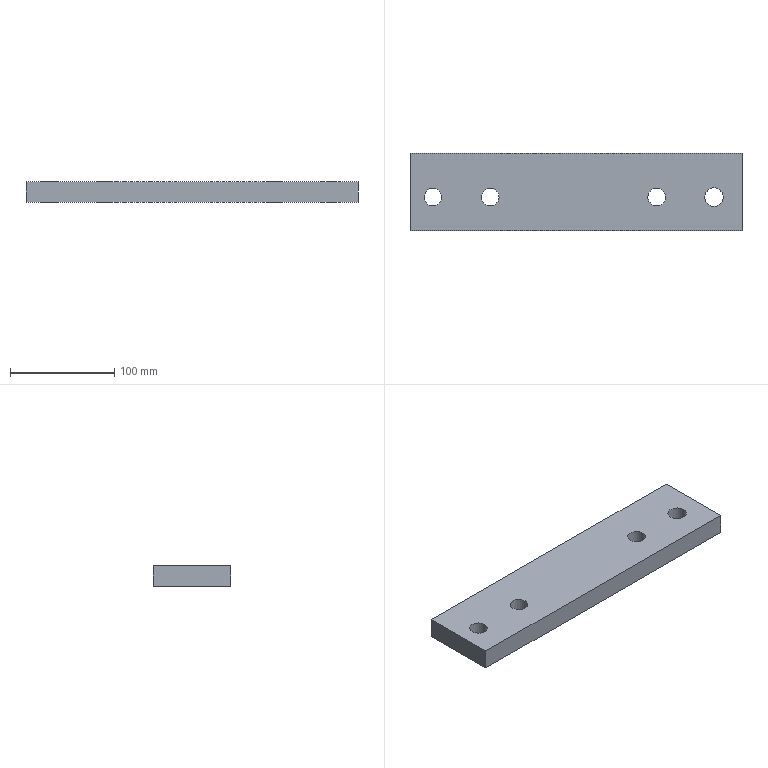Part | NX | features DATUM_CSYS 2, EXTRUDE 1, SKETCH 1 | 1 solid | 10 faces | box 319 x 74 x 20 mm | volume 453715 mm3 | plane 6 | cylinder 4 | commonest cylinder face diameters 16.87 x1 16.873 x1 16.982 x1 17.722 x1
STEP:
#1=CARTESIAN_POINT('',(-189.,-37.,0.));
#2=VERTEX_POINT('',#1);
#3=CARTESIAN_POINT('',(130.,-37.,0.));
#4=VERTEX_POINT('',#3);
#5=CARTESIAN_POINT('',(-189.,-37.,0.));
#6=DIRECTION('',(1.,0.,0.));
#7=VECTOR('',#6,1000.);
#8=LINE('',#5,#7);
#9=EDGE_CURVE('',#2,#4,#8,.T.);
#10=ORIENTED_EDGE('',*,*,#9,.T.);
#11=CARTESIAN_POINT('',(130.,-37.,20.));
#12=VERTEX_POINT('',#11);
#13=CARTESIAN_POINT('',(130.,-37.,20.));
#14=DIRECTION('',(0.,0.,-1.));
#15=VECTOR('',#14,1000.);
#16=LINE('',#13,#15);
#17=EDGE_CURVE('',#12,#4,#16,.T.);
#18=ORIENTED_EDGE('',*,*,#17,.F.);
#19=CARTESIAN_POINT('',(-189.,-37.,20.));
#20=VERTEX_POINT('',#19);
#21=CARTESIAN_POINT('',(-189.,-37.,20.));
#22=DIRECTION('',(1.,0.,0.));
#23=VECTOR('',#22,1000.);
#24=LINE('',#21,#23);
#25=EDGE_CURVE('',#20,#12,#24,.T.);
#26=ORIENTED_EDGE('',*,*,#25,.F.);
#27=CARTESIAN_POINT('',(-189.,-37.,20.));
#28=DIRECTION('',(0.,0.,-1.));
#29=VECTOR('',#28,1000.);
#30=LINE('',#27,#29);
#31=EDGE_CURVE('',#20,#2,#30,.T.);
#32=ORIENTED_EDGE('',*,*,#31,.T.);
#33=EDGE_LOOP('',(#10,#18,#26,#32));
#34=FACE_BOUND('',#33,.T.);
#35=CARTESIAN_POINT('',(-189.,-37.,20.));
#36=DIRECTION('',(0.,1.,0.));
#37=DIRECTION('',(0.,0.,1.));
#38=AXIS2_PLACEMENT_3D('',#35,#36,#37);
#39=PLANE('',#38);
#40=ADVANCED_FACE('',(#34),#39,.F.);
#41=CARTESIAN_POINT('',(130.,37.,0.));
#42=VERTEX_POINT('',#41);
#43=CARTESIAN_POINT('',(130.,-37.,0.));
#44=DIRECTION('',(0.,1.,0.));
#45=VECTOR('',#44,1000.);
#46=LINE('',#43,#45);
#47=EDGE_CURVE('',#4,#42,#46,.T.);
#48=ORIENTED_EDGE('',*,*,#47,.T.);
#49=CARTESIAN_POINT('',(130.,37.,20.));
#50=VERTEX_POINT('',#49);
#51=CARTESIAN_POINT('',(130.,37.,20.));
#52=DIRECTION('',(0.,0.,-1.));
#53=VECTOR('',#52,1000.);
#54=LINE('',#51,#53);
#55=EDGE_CURVE('',#50,#42,#54,.T.);
#56=ORIENTED_EDGE('',*,*,#55,.F.);
#57=CARTESIAN_POINT('',(130.,-37.,20.));
#58=DIRECTION('',(0.,1.,0.));
#59=VECTOR('',#58,1000.);
#60=LINE('',#57,#59);
#61=EDGE_CURVE('',#12,#50,#60,.T.);
#62=ORIENTED_EDGE('',*,*,#61,.F.);
#63=ORIENTED_EDGE('',*,*,#17,.T.);
#64=EDGE_LOOP('',(#48,#56,#62,#63));
#65=FACE_BOUND('',#64,.T.);
#66=CARTESIAN_POINT('',(130.,-37.,20.));
#67=DIRECTION('',(-1.,0.,0.));
#68=DIRECTION('',(0.,0.,1.));
#69=AXIS2_PLACEMENT_3D('',#66,#67,#68);
#70=PLANE('',#69);
#71=ADVANCED_FACE('',(#65),#70,.F.);
#72=CARTESIAN_POINT('',(-189.,37.,0.));
#73=VERTEX_POINT('',#72);
#74=CARTESIAN_POINT('',(130.,37.,0.));
#75=DIRECTION('',(-1.,0.,0.));
#76=VECTOR('',#75,1000.);
#77=LINE('',#74,#76);
#78=EDGE_CURVE('',#42,#73,#77,.T.);
#79=ORIENTED_EDGE('',*,*,#78,.T.);
#80=CARTESIAN_POINT('',(-189.,37.,20.));
#81=VERTEX_POINT('',#80);
#82=CARTESIAN_POINT('',(-189.,37.,20.));
#83=DIRECTION('',(0.,0.,-1.));
#84=VECTOR('',#83,1000.);
#85=LINE('',#82,#84);
#86=EDGE_CURVE('',#81,#73,#85,.T.);
#87=ORIENTED_EDGE('',*,*,#86,.F.);
#88=CARTESIAN_POINT('',(130.,37.,20.));
#89=DIRECTION('',(-1.,0.,0.));
#90=VECTOR('',#89,1000.);
#91=LINE('',#88,#90);
#92=EDGE_CURVE('',#50,#81,#91,.T.);
#93=ORIENTED_EDGE('',*,*,#92,.F.);
#94=ORIENTED_EDGE('',*,*,#55,.T.);
#95=EDGE_LOOP('',(#79,#87,#93,#94));
#96=FACE_BOUND('',#95,.T.);
#97=CARTESIAN_POINT('',(130.,37.,20.));
#98=DIRECTION('',(0.,-1.,0.));
#99=DIRECTION('',(0.,0.,-1.));
#100=AXIS2_PLACEMENT_3D('',#97,#98,#99);
#101=PLANE('',#100);
#102=ADVANCED_FACE('',(#96),#101,.F.);
#103=CARTESIAN_POINT('',(56.502,-4.93,20.));
#104=VERTEX_POINT('',#103);
#105=CARTESIAN_POINT('',(48.011,-4.93,20.));
#106=DIRECTION('',(0.,0.,1.));
#107=DIRECTION('',(1.,0.,0.));
#108=AXIS2_PLACEMENT_3D('',#105,#106,#107);
#109=CIRCLE('',#108,8.491);
#110=EDGE_CURVE('',#104,#104,#109,.T.);
#111=ORIENTED_EDGE('',*,*,#110,.T.);
#112=EDGE_LOOP('',(#111));
#113=FACE_BOUND('',#112,.T.);
#114=CARTESIAN_POINT('',(56.502,-4.93,0.));
#115=VERTEX_POINT('',#114);
#116=CARTESIAN_POINT('',(48.011,-4.93,0.));
#117=DIRECTION('',(0.,0.,1.));
#118=DIRECTION('',(1.,0.,0.));
#119=AXIS2_PLACEMENT_3D('',#116,#117,#118);
#120=CIRCLE('',#119,8.491);
#121=EDGE_CURVE('',#115,#115,#120,.T.);
#122=ORIENTED_EDGE('',*,*,#121,.F.);
#123=EDGE_LOOP('',(#122));
#124=FACE_BOUND('',#123,.T.);
#125=CARTESIAN_POINT('',(48.011,-4.93,20.));
#126=DIRECTION('',(0.,0.,-1.));
#127=DIRECTION('',(-1.,0.,0.));
#128=AXIS2_PLACEMENT_3D('',#125,#126,#127);
#129=CYLINDRICAL_SURFACE('',#128,8.491);
#130=ADVANCED_FACE('',(#113,#124),#129,.F.);
#131=CARTESIAN_POINT('',(-103.405,-4.93,20.));
#132=VERTEX_POINT('',#131);
#133=CARTESIAN_POINT('',(-111.841,-4.93,20.));
#134=DIRECTION('',(0.,0.,1.));
#135=DIRECTION('',(1.,0.,0.));
#136=AXIS2_PLACEMENT_3D('',#133,#134,#135);
#137=CIRCLE('',#136,8.436);
#138=EDGE_CURVE('',#132,#132,#137,.T.);
#139=ORIENTED_EDGE('',*,*,#138,.T.);
#140=EDGE_LOOP('',(#139));
#141=FACE_BOUND('',#140,.T.);
#142=CARTESIAN_POINT('',(-103.405,-4.93,0.));
#143=VERTEX_POINT('',#142);
#144=CARTESIAN_POINT('',(-111.841,-4.93,0.));
#145=DIRECTION('',(0.,0.,1.));
#146=DIRECTION('',(1.,0.,0.));
#147=AXIS2_PLACEMENT_3D('',#144,#145,#146);
#148=CIRCLE('',#147,8.436);
#149=EDGE_CURVE('',#143,#143,#148,.T.);
#150=ORIENTED_EDGE('',*,*,#149,.F.);
#151=EDGE_LOOP('',(#150));
#152=FACE_BOUND('',#151,.T.);
#153=CARTESIAN_POINT('',(-111.841,-4.93,20.));
#154=DIRECTION('',(0.,0.,-1.));
#155=DIRECTION('',(-1.,0.,0.));
#156=AXIS2_PLACEMENT_3D('',#153,#154,#155);
#157=CYLINDRICAL_SURFACE('',#156,8.436);
#158=ADVANCED_FACE('',(#141,#152),#157,.F.);
#159=CARTESIAN_POINT('',(-158.578,-4.93,20.));
#160=VERTEX_POINT('',#159);
#161=CARTESIAN_POINT('',(-167.013,-4.93,20.));
#162=DIRECTION('',(0.,0.,1.));
#163=DIRECTION('',(1.,0.,0.));
#164=AXIS2_PLACEMENT_3D('',#161,#162,#163);
#165=CIRCLE('',#164,8.435);
#166=EDGE_CURVE('',#160,#160,#165,.T.);
#167=ORIENTED_EDGE('',*,*,#166,.T.);
#168=EDGE_LOOP('',(#167));
#169=FACE_BOUND('',#168,.T.);
#170=CARTESIAN_POINT('',(-158.578,-4.93,0.));
#171=VERTEX_POINT('',#170);
#172=CARTESIAN_POINT('',(-167.013,-4.93,0.));
#173=DIRECTION('',(0.,0.,1.));
#174=DIRECTION('',(1.,0.,0.));
#175=AXIS2_PLACEMENT_3D('',#172,#173,#174);
#176=CIRCLE('',#175,8.435);
#177=EDGE_CURVE('',#171,#171,#176,.T.);
#178=ORIENTED_EDGE('',*,*,#177,.F.);
#179=EDGE_LOOP('',(#178));
#180=FACE_BOUND('',#179,.T.);
#181=CARTESIAN_POINT('',(-167.013,-4.93,20.));
#182=DIRECTION('',(0.,0.,-1.));
#183=DIRECTION('',(-1.,0.,0.));
#184=AXIS2_PLACEMENT_3D('',#181,#182,#183);
#185=CYLINDRICAL_SURFACE('',#184,8.435);
#186=ADVANCED_FACE('',(#169,#180),#185,.F.);
#187=CARTESIAN_POINT('',(-189.,37.,0.));
#188=DIRECTION('',(0.,-1.,0.));
#189=VECTOR('',#188,1000.);
#190=LINE('',#187,#189);
#191=EDGE_CURVE('',#73,#2,#190,.T.);
#192=ORIENTED_EDGE('',*,*,#191,.T.);
#193=ORIENTED_EDGE('',*,*,#31,.F.);
#194=CARTESIAN_POINT('',(-189.,37.,20.));
#195=DIRECTION('',(0.,-1.,0.));
#196=VECTOR('',#195,1000.);
#197=LINE('',#194,#196);
#198=EDGE_CURVE('',#81,#20,#197,.T.);
#199=ORIENTED_EDGE('',*,*,#198,.F.);
#200=ORIENTED_EDGE('',*,*,#86,.T.);
#201=EDGE_LOOP('',(#192,#193,#199,#200));
#202=FACE_BOUND('',#201,.T.);
#203=CARTESIAN_POINT('',(-189.,37.,20.));
#204=DIRECTION('',(1.,0.,0.));
#205=DIRECTION('',(0.,1.,0.));
#206=AXIS2_PLACEMENT_3D('',#203,#204,#205);
#207=PLANE('',#206);
#208=ADVANCED_FACE('',(#202),#207,.F.);
#209=CARTESIAN_POINT('',(111.917,-4.93,20.));
#210=VERTEX_POINT('',#209);
#211=CARTESIAN_POINT('',(103.056,-4.93,20.));
#212=DIRECTION('',(0.,0.,1.));
#213=DIRECTION('',(1.,0.,0.));
#214=AXIS2_PLACEMENT_3D('',#211,#212,#213);
#215=CIRCLE('',#214,8.861);
#216=EDGE_CURVE('',#210,#210,#215,.T.);
#217=ORIENTED_EDGE('',*,*,#216,.T.);
#218=EDGE_LOOP('',(#217));
#219=FACE_BOUND('',#218,.T.);
#220=CARTESIAN_POINT('',(111.917,-4.93,0.));
#221=VERTEX_POINT('',#220);
#222=CARTESIAN_POINT('',(103.056,-4.93,0.));
#223=DIRECTION('',(0.,0.,1.));
#224=DIRECTION('',(1.,0.,0.));
#225=AXIS2_PLACEMENT_3D('',#222,#223,#224);
#226=CIRCLE('',#225,8.861);
#227=EDGE_CURVE('',#221,#221,#226,.T.);
#228=ORIENTED_EDGE('',*,*,#227,.F.);
#229=EDGE_LOOP('',(#228));
#230=FACE_BOUND('',#229,.T.);
#231=CARTESIAN_POINT('',(103.056,-4.93,20.));
#232=DIRECTION('',(0.,0.,-1.));
#233=DIRECTION('',(-1.,0.,0.));
#234=AXIS2_PLACEMENT_3D('',#231,#232,#233);
#235=CYLINDRICAL_SURFACE('',#234,8.861);
#236=ADVANCED_FACE('',(#219,#230),#235,.F.);
#237=ORIENTED_EDGE('',*,*,#25,.T.);
#238=ORIENTED_EDGE('',*,*,#61,.T.);
#239=ORIENTED_EDGE('',*,*,#92,.T.);
#240=ORIENTED_EDGE('',*,*,#198,.T.);
#241=EDGE_LOOP('',(#237,#238,#239,#240));
#242=FACE_BOUND('',#241,.T.);
#243=ORIENTED_EDGE('',*,*,#166,.F.);
#244=EDGE_LOOP('',(#243));
#245=FACE_BOUND('',#244,.T.);
#246=ORIENTED_EDGE('',*,*,#138,.F.);
#247=EDGE_LOOP('',(#246));
#248=FACE_BOUND('',#247,.T.);
#249=ORIENTED_EDGE('',*,*,#110,.F.);
#250=EDGE_LOOP('',(#249));
#251=FACE_BOUND('',#250,.T.);
#252=ORIENTED_EDGE('',*,*,#216,.F.);
#253=EDGE_LOOP('',(#252));
#254=FACE_BOUND('',#253,.T.);
#255=CARTESIAN_POINT('',(-167.013,-4.93,20.));
#256=DIRECTION('',(0.,0.,1.));
#257=DIRECTION('',(1.,0.,0.));
#258=AXIS2_PLACEMENT_3D('',#255,#256,#257);
#259=PLANE('',#258);
#260=ADVANCED_FACE('',(#242,#245,#248,#251,#254),#259,.T.);
#261=ORIENTED_EDGE('',*,*,#9,.F.);
#262=ORIENTED_EDGE('',*,*,#191,.F.);
#263=ORIENTED_EDGE('',*,*,#78,.F.);
#264=ORIENTED_EDGE('',*,*,#47,.F.);
#265=EDGE_LOOP('',(#261,#262,#263,#264));
#266=FACE_BOUND('',#265,.T.);
#267=ORIENTED_EDGE('',*,*,#177,.T.);
#268=EDGE_LOOP('',(#267));
#269=FACE_BOUND('',#268,.T.);
#270=ORIENTED_EDGE('',*,*,#149,.T.);
#271=EDGE_LOOP('',(#270));
#272=FACE_BOUND('',#271,.T.);
#273=ORIENTED_EDGE('',*,*,#121,.T.);
#274=EDGE_LOOP('',(#273));
#275=FACE_BOUND('',#274,.T.);
#276=ORIENTED_EDGE('',*,*,#227,.T.);
#277=EDGE_LOOP('',(#276));
#278=FACE_BOUND('',#277,.T.);
#279=CARTESIAN_POINT('',(-167.013,-4.93,0.));
#280=DIRECTION('',(0.,0.,1.));
#281=DIRECTION('',(1.,0.,0.));
#282=AXIS2_PLACEMENT_3D('',#279,#280,#281);
#283=PLANE('',#282);
#284=ADVANCED_FACE('',(#266,#269,#272,#275,#278),#283,.F.);
#285=CLOSED_SHELL('',(#40,#71,#102,#130,#158,#186,#208,#236,#260,#284));
#286=MANIFOLD_SOLID_BREP('',#285);
#287=(LENGTH_UNIT()NAMED_UNIT(*)SI_UNIT(.MILLI.,.METRE.));
#288=UNCERTAINTY_MEASURE_WITH_UNIT(LENGTH_MEASURE(0.00001),#287,'','');
#289=(NAMED_UNIT(*)PLANE_ANGLE_UNIT()SI_UNIT($,.RADIAN.));
#290=(NAMED_UNIT(*)SI_UNIT($,.STERADIAN.)SOLID_ANGLE_UNIT());
#291=(GEOMETRIC_REPRESENTATION_CONTEXT(3)GLOBAL_UNCERTAINTY_ASSIGNED_CONTEXT((#288))GLOBAL_UNIT_ASSIGNED_CONTEXT((#287,#289,#290))REPRESENTATION_CONTEXT('',''));
#292=ADVANCED_BREP_SHAPE_REPRESENTATION('',(#286),#291);